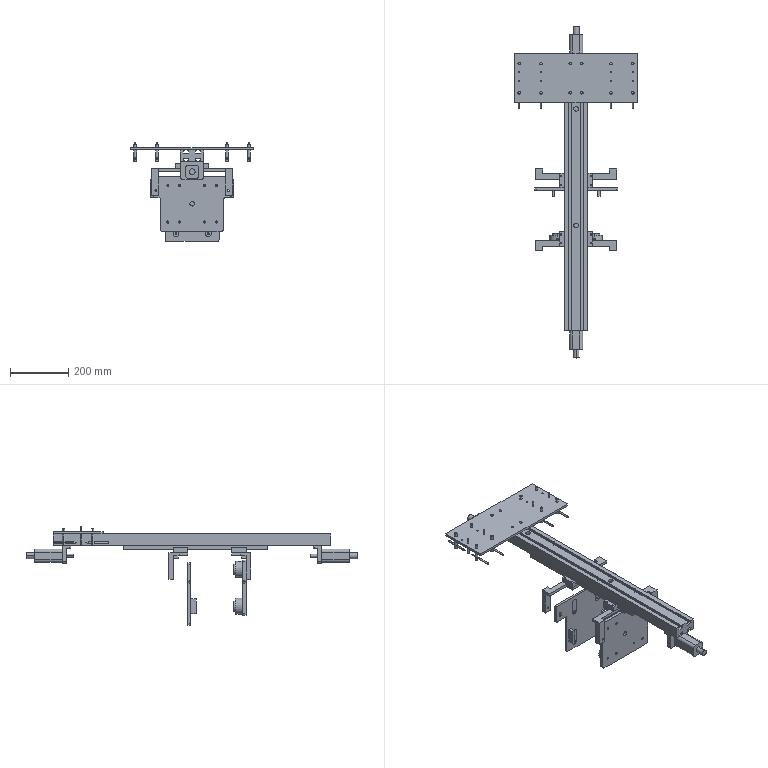Part | 48 solids | 1700 faces | box 420 x 1138 x 338.748 mm | volume 5232441 mm3 | plane 743 | cylinder 562 | spline 287 | cone 108 | commonest cylinder face diameters 5 x112 3.3 x56 6 x48 10 x44 5.5 x40 3.641 x32